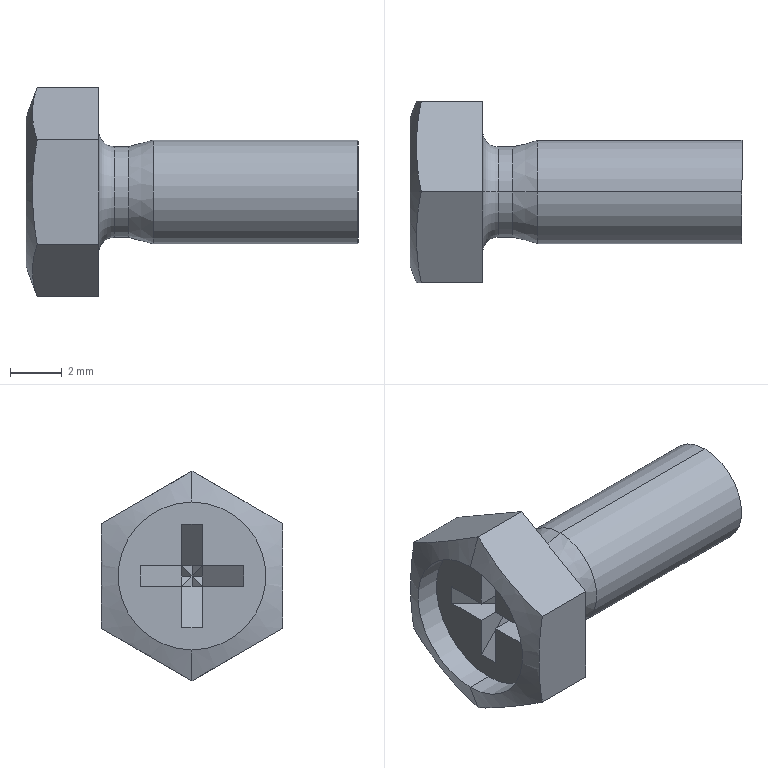Part | NX | features BREP 1 | 1 solid | 45 faces | box 12.8 x 7 x 8.083 mm | volume 207.191 mm3 | plane 33 | cylinder 6 | cone 4 | torus 2 | commonest cylinder face diameters 3.5 x2 4 x2 5.7 x2
STEP:
#1=CARTESIAN_POINT('',(1.,0.,-2.85));
#2=VERTEX_POINT('',#1);
#3=CARTESIAN_POINT('',(1.,0.,2.85));
#4=VERTEX_POINT('',#3);
#5=CARTESIAN_POINT('',(1.,0.,0.));
#6=DIRECTION('',(-1.,0.,0.));
#7=DIRECTION('',(0.,0.,1.));
#8=AXIS2_PLACEMENT_3D('',#5,#6,#7);
#9=CIRCLE('',#8,2.85);
#10=EDGE_CURVE('',#2,#4,#9,.T.);
#11=ORIENTED_EDGE('',*,*,#10,.F.);
#12=CARTESIAN_POINT('',(0.,0.,-2.85));
#13=VERTEX_POINT('',#12);
#14=CARTESIAN_POINT('',(1.,0.,-2.85));
#15=DIRECTION('',(-1.,0.,0.));
#16=VECTOR('',#15,1000.);
#17=LINE('',#14,#16);
#18=EDGE_CURVE('',#2,#13,#17,.T.);
#19=ORIENTED_EDGE('',*,*,#18,.T.);
#20=CARTESIAN_POINT('',(0.,0.,2.85));
#21=VERTEX_POINT('',#20);
#22=CARTESIAN_POINT('',(0.,0.,0.));
#23=DIRECTION('',(-1.,0.,0.));
#24=DIRECTION('',(0.,0.,1.));
#25=AXIS2_PLACEMENT_3D('',#22,#23,#24);
#26=CIRCLE('',#25,2.85);
#27=EDGE_CURVE('',#13,#21,#26,.T.);
#28=ORIENTED_EDGE('',*,*,#27,.T.);
#29=CARTESIAN_POINT('',(1.,0.,2.85));
#30=DIRECTION('',(-1.,0.,0.));
#31=VECTOR('',#30,1000.);
#32=LINE('',#29,#31);
#33=EDGE_CURVE('',#4,#21,#32,.T.);
#34=ORIENTED_EDGE('',*,*,#33,.F.);
#35=EDGE_LOOP('',(#11,#19,#28,#34));
#36=FACE_BOUND('',#35,.T.);
#37=CARTESIAN_POINT('',(1.,0.,0.));
#38=DIRECTION('',(-1.,0.,0.));
#39=DIRECTION('',(0.,0.,1.));
#40=AXIS2_PLACEMENT_3D('',#37,#38,#39);
#41=CYLINDRICAL_SURFACE('',#40,2.85);
#42=ADVANCED_FACE('',(#36),#41,.F.);
#43=CARTESIAN_POINT('',(1.,0.,0.));
#44=DIRECTION('',(-1.,0.,0.));
#45=DIRECTION('',(0.,0.,1.));
#46=AXIS2_PLACEMENT_3D('',#43,#44,#45);
#47=CIRCLE('',#46,2.85);
#48=EDGE_CURVE('',#4,#2,#47,.T.);
#49=ORIENTED_EDGE('',*,*,#48,.T.);
#50=ORIENTED_EDGE('',*,*,#10,.T.);
#51=EDGE_LOOP('',(#49,#50));
#52=FACE_BOUND('',#51,.T.);
#53=CARTESIAN_POINT('',(1.,2.,0.386));
#54=VERTEX_POINT('',#53);
#55=CARTESIAN_POINT('',(1.,2.,-0.386));
#56=VERTEX_POINT('',#55);
#57=CARTESIAN_POINT('',(1.,2.,0.));
#58=DIRECTION('',(0.,0.,-1.));
#59=VECTOR('',#58,1000.);
#60=LINE('',#57,#59);
#61=EDGE_CURVE('',#54,#56,#60,.T.);
#62=ORIENTED_EDGE('',*,*,#61,.F.);
#63=CARTESIAN_POINT('',(1.,0.386,0.386));
#64=VERTEX_POINT('',#63);
#65=CARTESIAN_POINT('',(1.,1.193,0.386));
#66=DIRECTION('',(0.,-1.,0.));
#67=VECTOR('',#66,1000.);
#68=LINE('',#65,#67);
#69=EDGE_CURVE('',#54,#64,#68,.T.);
#70=ORIENTED_EDGE('',*,*,#69,.T.);
#71=CARTESIAN_POINT('',(1.,0.386,2.));
#72=VERTEX_POINT('',#71);
#73=CARTESIAN_POINT('',(1.,0.386,1.193));
#74=DIRECTION('',(0.,0.,-1.));
#75=VECTOR('',#74,1000.);
#76=LINE('',#73,#75);
#77=EDGE_CURVE('',#72,#64,#76,.T.);
#78=ORIENTED_EDGE('',*,*,#77,.F.);
#79=CARTESIAN_POINT('',(1.,-0.386,2.));
#80=VERTEX_POINT('',#79);
#81=CARTESIAN_POINT('',(1.,0.,2.));
#82=DIRECTION('',(0.,1.,0.));
#83=VECTOR('',#82,1000.);
#84=LINE('',#81,#83);
#85=EDGE_CURVE('',#80,#72,#84,.T.);
#86=ORIENTED_EDGE('',*,*,#85,.F.);
#87=CARTESIAN_POINT('',(1.,-0.386,0.386));
#88=VERTEX_POINT('',#87);
#89=CARTESIAN_POINT('',(1.,-0.386,1.193));
#90=DIRECTION('',(0.,0.,-1.));
#91=VECTOR('',#90,1000.);
#92=LINE('',#89,#91);
#93=EDGE_CURVE('',#80,#88,#92,.T.);
#94=ORIENTED_EDGE('',*,*,#93,.T.);
#95=CARTESIAN_POINT('',(1.,-2.,0.386));
#96=VERTEX_POINT('',#95);
#97=CARTESIAN_POINT('',(1.,-1.193,0.386));
#98=DIRECTION('',(0.,-1.,0.));
#99=VECTOR('',#98,1000.);
#100=LINE('',#97,#99);
#101=EDGE_CURVE('',#88,#96,#100,.T.);
#102=ORIENTED_EDGE('',*,*,#101,.T.);
#103=CARTESIAN_POINT('',(1.,-2.,-0.386));
#104=VERTEX_POINT('',#103);
#105=CARTESIAN_POINT('',(1.,-2.,0.));
#106=DIRECTION('',(0.,0.,1.));
#107=VECTOR('',#106,1000.);
#108=LINE('',#105,#107);
#109=EDGE_CURVE('',#104,#96,#108,.T.);
#110=ORIENTED_EDGE('',*,*,#109,.F.);
#111=CARTESIAN_POINT('',(1.,-0.386,-0.386));
#112=VERTEX_POINT('',#111);
#113=CARTESIAN_POINT('',(1.,-1.193,-0.386));
#114=DIRECTION('',(0.,-1.,0.));
#115=VECTOR('',#114,1000.);
#116=LINE('',#113,#115);
#117=EDGE_CURVE('',#112,#104,#116,.T.);
#118=ORIENTED_EDGE('',*,*,#117,.F.);
#119=CARTESIAN_POINT('',(1.,-0.386,-2.));
#120=VERTEX_POINT('',#119);
#121=CARTESIAN_POINT('',(1.,-0.386,-1.193));
#122=DIRECTION('',(0.,0.,-1.));
#123=VECTOR('',#122,1000.);
#124=LINE('',#121,#123);
#125=EDGE_CURVE('',#112,#120,#124,.T.);
#126=ORIENTED_EDGE('',*,*,#125,.T.);
#127=CARTESIAN_POINT('',(1.,0.386,-2.));
#128=VERTEX_POINT('',#127);
#129=CARTESIAN_POINT('',(1.,0.,-2.));
#130=DIRECTION('',(0.,-1.,0.));
#131=VECTOR('',#130,1000.);
#132=LINE('',#129,#131);
#133=EDGE_CURVE('',#128,#120,#132,.T.);
#134=ORIENTED_EDGE('',*,*,#133,.F.);
#135=CARTESIAN_POINT('',(1.,0.386,-0.386));
#136=VERTEX_POINT('',#135);
#137=CARTESIAN_POINT('',(1.,0.386,-1.193));
#138=DIRECTION('',(0.,0.,-1.));
#139=VECTOR('',#138,1000.);
#140=LINE('',#137,#139);
#141=EDGE_CURVE('',#136,#128,#140,.T.);
#142=ORIENTED_EDGE('',*,*,#141,.F.);
#143=CARTESIAN_POINT('',(1.,1.193,-0.386));
#144=DIRECTION('',(0.,-1.,0.));
#145=VECTOR('',#144,1000.);
#146=LINE('',#143,#145);
#147=EDGE_CURVE('',#56,#136,#146,.T.);
#148=ORIENTED_EDGE('',*,*,#147,.F.);
#149=EDGE_LOOP('',(#62,#70,#78,#86,#94,#102,#110,#118,#126,#134,#142,#148));
#150=FACE_BOUND('',#149,.T.);
#151=CARTESIAN_POINT('',(1.,0.,0.));
#152=DIRECTION('',(-1.,0.,0.));
#153=DIRECTION('',(0.,0.,-1.));
#154=AXIS2_PLACEMENT_3D('',#151,#152,#153);
#155=PLANE('',#154);
#156=ADVANCED_FACE('',(#52,#150),#155,.T.);
#157=ORIENTED_EDGE('',*,*,#18,.F.);
#158=ORIENTED_EDGE('',*,*,#48,.F.);
#159=ORIENTED_EDGE('',*,*,#33,.T.);
#160=CARTESIAN_POINT('',(0.,0.,0.));
#161=DIRECTION('',(-1.,0.,0.));
#162=DIRECTION('',(0.,0.,1.));
#163=AXIS2_PLACEMENT_3D('',#160,#161,#162);
#164=CIRCLE('',#163,2.85);
#165=EDGE_CURVE('',#21,#13,#164,.T.);
#166=ORIENTED_EDGE('',*,*,#165,.T.);
#167=EDGE_LOOP('',(#157,#158,#159,#166));
#168=FACE_BOUND('',#167,.T.);
#169=CARTESIAN_POINT('',(1.,0.,0.));
#170=DIRECTION('',(-1.,0.,0.));
#171=DIRECTION('',(0.,0.,-1.));
#172=AXIS2_PLACEMENT_3D('',#169,#170,#171);
#173=CYLINDRICAL_SURFACE('',#172,2.85);
#174=ADVANCED_FACE('',(#168),#173,.F.);
#175=CARTESIAN_POINT('',(0.4337,0.000000012,4.041));
#176=VERTEX_POINT('',#175);
#177=CARTESIAN_POINT('',(171009.553,0.,469847.735));
#178=DIRECTION('',(0.342,0.,0.9397));
#179=VECTOR('',#178,1000.);
#180=LINE('',#177,#179);
#181=EDGE_CURVE('',#21,#176,#180,.T.);
#182=ORIENTED_EDGE('',*,*,#181,.F.);
#183=ORIENTED_EDGE('',*,*,#27,.F.);
#184=CARTESIAN_POINT('',(0.4337,0.000000012,-4.041));
#185=VERTEX_POINT('',#184);
#186=CARTESIAN_POINT('',(171009.553,0.,-469847.735));
#187=DIRECTION('',(0.342,0.,-0.9397));
#188=VECTOR('',#187,1000.);
#189=LINE('',#186,#188);
#190=EDGE_CURVE('',#13,#185,#189,.T.);
#191=ORIENTED_EDGE('',*,*,#190,.T.);
#192=CARTESIAN_POINT('',(0.4337,-3.5,-2.021));
#193=VERTEX_POINT('',#192);
#194=CARTESIAN_POINT('',(0.4337,-0.000000048,-4.041));
#195=CARTESIAN_POINT('',(0.1885,-1.167,-3.368));
#196=CARTESIAN_POINT('',(0.1885,-2.333,-2.694));
#197=CARTESIAN_POINT('',(0.4337,-3.5,-2.021));
#198=B_SPLINE_CURVE_WITH_KNOTS('',3,(#194,#195,#196,#197),.UNSPECIFIED.,.F.,.F.,(4,4),(0.,0.004041),.UNSPECIFIED.);
#199=EDGE_CURVE('',#185,#193,#198,.T.);
#200=ORIENTED_EDGE('',*,*,#199,.T.);
#201=CARTESIAN_POINT('',(0.4337,-3.5,2.021));
#202=VERTEX_POINT('',#201);
#203=CARTESIAN_POINT('',(0.4337,-3.5,-2.021));
#204=CARTESIAN_POINT('',(0.1885,-3.5,-0.6736));
#205=CARTESIAN_POINT('',(0.1885,-3.5,0.6736));
#206=CARTESIAN_POINT('',(0.4337,-3.5,2.021));
#207=B_SPLINE_CURVE_WITH_KNOTS('',3,(#203,#204,#205,#206),.UNSPECIFIED.,.F.,.F.,(4,4),(0.,0.004041),.UNSPECIFIED.);
#208=EDGE_CURVE('',#193,#202,#207,.T.);
#209=ORIENTED_EDGE('',*,*,#208,.T.);
#210=CARTESIAN_POINT('',(0.4337,-3.5,2.021));
#211=CARTESIAN_POINT('',(0.1885,-2.333,2.694));
#212=CARTESIAN_POINT('',(0.1885,-1.167,3.368));
#213=CARTESIAN_POINT('',(0.4337,-0.000000025,4.041));
#214=B_SPLINE_CURVE_WITH_KNOTS('',3,(#210,#211,#212,#213),.UNSPECIFIED.,.F.,.F.,(4,4),(0.,0.004041),.UNSPECIFIED.);
#215=EDGE_CURVE('',#202,#176,#214,.T.);
#216=ORIENTED_EDGE('',*,*,#215,.T.);
#217=EDGE_LOOP('',(#182,#183,#191,#200,#209,#216));
#218=FACE_BOUND('',#217,.T.);
#219=CARTESIAN_POINT('',(0.,0.,0.));
#220=DIRECTION('',(1.,0.,0.));
#221=DIRECTION('',(0.,0.,-1.));
#222=AXIS2_PLACEMENT_3D('',#219,#220,#221);
#223=CONICAL_SURFACE('',#222,2.85,1.222);
#224=ADVANCED_FACE('',(#218),#223,.T.);
#225=ORIENTED_EDGE('',*,*,#61,.T.);
#226=CARTESIAN_POINT('',(2.558,0.386,-0.386));
#227=VERTEX_POINT('',#226);
#228=CARTESIAN_POINT('',(1.779,1.193,-0.386));
#229=DIRECTION('',(0.6944,-0.7196,0.));
#230=VECTOR('',#229,1000.);
#231=LINE('',#228,#230);
#232=EDGE_CURVE('',#56,#227,#231,.T.);
#233=ORIENTED_EDGE('',*,*,#232,.T.);
#234=CARTESIAN_POINT('',(2.558,0.386,0.386));
#235=VERTEX_POINT('',#234);
#236=CARTESIAN_POINT('',(2.558,0.386,0.));
#237=DIRECTION('',(0.,0.,-1.));
#238=VECTOR('',#237,1000.);
#239=LINE('',#236,#238);
#240=EDGE_CURVE('',#235,#227,#239,.T.);
#241=ORIENTED_EDGE('',*,*,#240,.F.);
#242=CARTESIAN_POINT('',(1.779,1.193,0.386));
#243=DIRECTION('',(0.6944,-0.7196,0.));
#244=VECTOR('',#243,1000.);
#245=LINE('',#242,#244);
#246=EDGE_CURVE('',#54,#235,#245,.T.);
#247=ORIENTED_EDGE('',*,*,#246,.F.);
#248=EDGE_LOOP('',(#225,#233,#241,#247));
#249=FACE_BOUND('',#248,.T.);
#250=CARTESIAN_POINT('',(0.5,2.518,0.386));
#251=DIRECTION('',(0.7196,0.6944,0.));
#252=DIRECTION('',(0.6944,-0.7196,0.));
#253=AXIS2_PLACEMENT_3D('',#250,#251,#252);
#254=PLANE('',#253);
#255=ADVANCED_FACE('',(#249),#254,.F.);
#256=ORIENTED_EDGE('',*,*,#246,.T.);
#257=CARTESIAN_POINT('',(1.779,0.386,0.386));
#258=DIRECTION('',(-1.,0.,0.));
#259=VECTOR('',#258,1000.);
#260=LINE('',#257,#259);
#261=EDGE_CURVE('',#235,#64,#260,.T.);
#262=ORIENTED_EDGE('',*,*,#261,.T.);
#263=ORIENTED_EDGE('',*,*,#69,.F.);
#264=EDGE_LOOP('',(#256,#262,#263));
#265=FACE_BOUND('',#264,.T.);
#266=CARTESIAN_POINT('',(2.93,0.,0.386));
#267=DIRECTION('',(0.,0.,-1.));
#268=DIRECTION('',(0.,-1.,0.));
#269=AXIS2_PLACEMENT_3D('',#266,#267,#268);
#270=PLANE('',#269);
#271=ADVANCED_FACE('',(#265),#270,.T.);
#272=ORIENTED_EDGE('',*,*,#261,.F.);
#273=CARTESIAN_POINT('',(1.779,0.386,1.193));
#274=DIRECTION('',(0.6944,0.,-0.7196));
#275=VECTOR('',#274,1000.);
#276=LINE('',#273,#275);
#277=EDGE_CURVE('',#72,#235,#276,.T.);
#278=ORIENTED_EDGE('',*,*,#277,.F.);
#279=ORIENTED_EDGE('',*,*,#77,.T.);
#280=EDGE_LOOP('',(#272,#278,#279));
#281=FACE_BOUND('',#280,.T.);
#282=CARTESIAN_POINT('',(2.93,0.386,0.));
#283=DIRECTION('',(0.,1.,0.));
#284=DIRECTION('',(0.,0.,-1.));
#285=AXIS2_PLACEMENT_3D('',#282,#283,#284);
#286=PLANE('',#285);
#287=ADVANCED_FACE('',(#281),#286,.F.);
#288=CARTESIAN_POINT('',(2.558,-0.386,0.386));
#289=VERTEX_POINT('',#288);
#290=CARTESIAN_POINT('',(2.558,0.,0.386));
#291=DIRECTION('',(0.,1.,0.));
#292=VECTOR('',#291,1000.);
#293=LINE('',#290,#292);
#294=EDGE_CURVE('',#289,#235,#293,.T.);
#295=ORIENTED_EDGE('',*,*,#294,.F.);
#296=CARTESIAN_POINT('',(1.779,-0.386,1.193));
#297=DIRECTION('',(0.6944,0.,-0.7196));
#298=VECTOR('',#297,1000.);
#299=LINE('',#296,#298);
#300=EDGE_CURVE('',#80,#289,#299,.T.);
#301=ORIENTED_EDGE('',*,*,#300,.F.);
#302=ORIENTED_EDGE('',*,*,#85,.T.);
#303=ORIENTED_EDGE('',*,*,#277,.T.);
#304=EDGE_LOOP('',(#295,#301,#302,#303));
#305=FACE_BOUND('',#304,.T.);
#306=CARTESIAN_POINT('',(0.5,-0.386,2.518));
#307=DIRECTION('',(0.7196,0.,0.6944));
#308=DIRECTION('',(-0.6944,0.,0.7196));
#309=AXIS2_PLACEMENT_3D('',#306,#307,#308);
#310=PLANE('',#309);
#311=ADVANCED_FACE('',(#305),#310,.F.);
#312=ORIENTED_EDGE('',*,*,#300,.T.);
#313=CARTESIAN_POINT('',(1.779,-0.386,0.386));
#314=DIRECTION('',(-1.,0.,0.));
#315=VECTOR('',#314,1000.);
#316=LINE('',#313,#315);
#317=EDGE_CURVE('',#289,#88,#316,.T.);
#318=ORIENTED_EDGE('',*,*,#317,.T.);
#319=ORIENTED_EDGE('',*,*,#93,.F.);
#320=EDGE_LOOP('',(#312,#318,#319));
#321=FACE_BOUND('',#320,.T.);
#322=CARTESIAN_POINT('',(2.93,-0.386,0.));
#323=DIRECTION('',(0.,1.,0.));
#324=DIRECTION('',(0.,0.,-1.));
#325=AXIS2_PLACEMENT_3D('',#322,#323,#324);
#326=PLANE('',#325);
#327=ADVANCED_FACE('',(#321),#326,.T.);
#328=ORIENTED_EDGE('',*,*,#317,.F.);
#329=CARTESIAN_POINT('',(1.779,-1.193,0.386));
#330=DIRECTION('',(-0.6944,-0.7196,0.));
#331=VECTOR('',#330,1000.);
#332=LINE('',#329,#331);
#333=EDGE_CURVE('',#289,#96,#332,.T.);
#334=ORIENTED_EDGE('',*,*,#333,.T.);
#335=ORIENTED_EDGE('',*,*,#101,.F.);
#336=EDGE_LOOP('',(#328,#334,#335));
#337=FACE_BOUND('',#336,.T.);
#338=CARTESIAN_POINT('',(2.93,0.,0.386));
#339=DIRECTION('',(0.,0.,-1.));
#340=DIRECTION('',(0.,-1.,0.));
#341=AXIS2_PLACEMENT_3D('',#338,#339,#340);
#342=PLANE('',#341);
#343=ADVANCED_FACE('',(#337),#342,.T.);
#344=ORIENTED_EDGE('',*,*,#109,.T.);
#345=ORIENTED_EDGE('',*,*,#333,.F.);
#346=CARTESIAN_POINT('',(2.558,-0.386,-0.386));
#347=VERTEX_POINT('',#346);
#348=CARTESIAN_POINT('',(2.558,-0.386,0.));
#349=DIRECTION('',(0.,0.,-1.));
#350=VECTOR('',#349,1000.);
#351=LINE('',#348,#350);
#352=EDGE_CURVE('',#289,#347,#351,.T.);
#353=ORIENTED_EDGE('',*,*,#352,.T.);
#354=CARTESIAN_POINT('',(1.779,-1.193,-0.386));
#355=DIRECTION('',(-0.6944,-0.7196,0.));
#356=VECTOR('',#355,1000.);
#357=LINE('',#354,#356);
#358=EDGE_CURVE('',#347,#104,#357,.T.);
#359=ORIENTED_EDGE('',*,*,#358,.T.);
#360=EDGE_LOOP('',(#344,#345,#353,#359));
#361=FACE_BOUND('',#360,.T.);
#362=CARTESIAN_POINT('',(2.93,0.,0.386));
#363=DIRECTION('',(0.7196,-0.6944,0.));
#364=DIRECTION('',(-0.6944,-0.7196,0.));
#365=AXIS2_PLACEMENT_3D('',#362,#363,#364);
#366=PLANE('',#365);
#367=ADVANCED_FACE('',(#361),#366,.F.);
#368=ORIENTED_EDGE('',*,*,#117,.T.);
#369=ORIENTED_EDGE('',*,*,#358,.F.);
#370=CARTESIAN_POINT('',(1.779,-0.386,-0.386));
#371=DIRECTION('',(-1.,0.,0.));
#372=VECTOR('',#371,1000.);
#373=LINE('',#370,#372);
#374=EDGE_CURVE('',#347,#112,#373,.T.);
#375=ORIENTED_EDGE('',*,*,#374,.T.);
#376=EDGE_LOOP('',(#368,#369,#375));
#377=FACE_BOUND('',#376,.T.);
#378=CARTESIAN_POINT('',(2.93,0.,-0.386));
#379=DIRECTION('',(0.,0.,-1.));
#380=DIRECTION('',(0.,-1.,0.));
#381=AXIS2_PLACEMENT_3D('',#378,#379,#380);
#382=PLANE('',#381);
#383=ADVANCED_FACE('',(#377),#382,.F.);
#384=ORIENTED_EDGE('',*,*,#374,.F.);
#385=CARTESIAN_POINT('',(1.779,-0.386,-1.193));
#386=DIRECTION('',(-0.6944,0.,-0.7196));
#387=VECTOR('',#386,1000.);
#388=LINE('',#385,#387);
#389=EDGE_CURVE('',#347,#120,#388,.T.);
#390=ORIENTED_EDGE('',*,*,#389,.T.);
#391=ORIENTED_EDGE('',*,*,#125,.F.);
#392=EDGE_LOOP('',(#384,#390,#391));
#393=FACE_BOUND('',#392,.T.);
#394=CARTESIAN_POINT('',(2.93,-0.386,0.));
#395=DIRECTION('',(0.,1.,0.));
#396=DIRECTION('',(0.,0.,-1.));
#397=AXIS2_PLACEMENT_3D('',#394,#395,#396);
#398=PLANE('',#397);
#399=ADVANCED_FACE('',(#393),#398,.T.);
#400=ORIENTED_EDGE('',*,*,#389,.F.);
#401=CARTESIAN_POINT('',(2.558,0.,-0.386));
#402=DIRECTION('',(0.,1.,0.));
#403=VECTOR('',#402,1000.);
#404=LINE('',#401,#403);
#405=EDGE_CURVE('',#347,#227,#404,.T.);
#406=ORIENTED_EDGE('',*,*,#405,.T.);
#407=CARTESIAN_POINT('',(1.779,0.386,-1.193));
#408=DIRECTION('',(-0.6944,0.,-0.7196));
#409=VECTOR('',#408,1000.);
#410=LINE('',#407,#409);
#411=EDGE_CURVE('',#227,#128,#410,.T.);
#412=ORIENTED_EDGE('',*,*,#411,.T.);
#413=ORIENTED_EDGE('',*,*,#133,.T.);
#414=EDGE_LOOP('',(#400,#406,#412,#413));
#415=FACE_BOUND('',#414,.T.);
#416=CARTESIAN_POINT('',(2.93,-0.386,0.));
#417=DIRECTION('',(0.7196,0.,-0.6944));
#418=DIRECTION('',(0.6944,0.,0.7196));
#419=AXIS2_PLACEMENT_3D('',#416,#417,#418);
#420=PLANE('',#419);
#421=ADVANCED_FACE('',(#415),#420,.F.);
#422=ORIENTED_EDGE('',*,*,#411,.F.);
#423=CARTESIAN_POINT('',(1.779,0.386,-0.386));
#424=DIRECTION('',(-1.,0.,0.));
#425=VECTOR('',#424,1000.);
#426=LINE('',#423,#425);
#427=EDGE_CURVE('',#227,#136,#426,.T.);
#428=ORIENTED_EDGE('',*,*,#427,.T.);
#429=ORIENTED_EDGE('',*,*,#141,.T.);
#430=EDGE_LOOP('',(#422,#428,#429));
#431=FACE_BOUND('',#430,.T.);
#432=CARTESIAN_POINT('',(2.93,0.386,0.));
#433=DIRECTION('',(0.,1.,0.));
#434=DIRECTION('',(0.,0.,-1.));
#435=AXIS2_PLACEMENT_3D('',#432,#433,#434);
#436=PLANE('',#435);
#437=ADVANCED_FACE('',(#431),#436,.F.);
#438=ORIENTED_EDGE('',*,*,#147,.T.);
#439=ORIENTED_EDGE('',*,*,#427,.F.);
#440=ORIENTED_EDGE('',*,*,#232,.F.);
#441=EDGE_LOOP('',(#438,#439,#440));
#442=FACE_BOUND('',#441,.T.);
#443=CARTESIAN_POINT('',(2.93,0.,-0.386));
#444=DIRECTION('',(0.,0.,-1.));
#445=DIRECTION('',(0.,-1.,0.));
#446=AXIS2_PLACEMENT_3D('',#443,#444,#445);
#447=PLANE('',#446);
#448=ADVANCED_FACE('',(#442),#447,.F.);
#449=ORIENTED_EDGE('',*,*,#165,.F.);
#450=ORIENTED_EDGE('',*,*,#181,.T.);
#451=CARTESIAN_POINT('',(0.4337,3.5,2.021));
#452=VERTEX_POINT('',#451);
#453=CARTESIAN_POINT('',(0.4337,0.000000059,4.041));
#454=CARTESIAN_POINT('',(0.1885,1.167,3.368));
#455=CARTESIAN_POINT('',(0.1885,2.333,2.694));
#456=CARTESIAN_POINT('',(0.4337,3.5,2.021));
#457=B_SPLINE_CURVE_WITH_KNOTS('',3,(#453,#454,#455,#456),.UNSPECIFIED.,.F.,.F.,(4,4),(0.,0.004041),.UNSPECIFIED.);
#458=EDGE_CURVE('',#176,#452,#457,.T.);
#459=ORIENTED_EDGE('',*,*,#458,.T.);
#460=CARTESIAN_POINT('',(0.4337,3.5,-2.021));
#461=VERTEX_POINT('',#460);
#462=CARTESIAN_POINT('',(0.4337,3.5,2.021));
#463=CARTESIAN_POINT('',(0.1885,3.5,0.6736));
#464=CARTESIAN_POINT('',(0.1885,3.5,-0.6736));
#465=CARTESIAN_POINT('',(0.4337,3.5,-2.021));
#466=B_SPLINE_CURVE_WITH_KNOTS('',3,(#462,#463,#464,#465),.UNSPECIFIED.,.F.,.F.,(4,4),(0.,0.004041),.UNSPECIFIED.);
#467=EDGE_CURVE('',#452,#461,#466,.T.);
#468=ORIENTED_EDGE('',*,*,#467,.T.);
#469=CARTESIAN_POINT('',(0.4337,3.5,-2.021));
#470=CARTESIAN_POINT('',(0.1885,2.333,-2.694));
#471=CARTESIAN_POINT('',(0.1885,1.167,-3.368));
#472=CARTESIAN_POINT('',(0.4337,0.000000003,-4.041));
#473=B_SPLINE_CURVE_WITH_KNOTS('',3,(#469,#470,#471,#472),.UNSPECIFIED.,.F.,.F.,(4,4),(0.,0.004041),.UNSPECIFIED.);
#474=EDGE_CURVE('',#461,#185,#473,.T.);
#475=ORIENTED_EDGE('',*,*,#474,.T.);
#476=ORIENTED_EDGE('',*,*,#190,.F.);
#477=EDGE_LOOP('',(#449,#450,#459,#468,#475,#476));
#478=FACE_BOUND('',#477,.T.);
#479=CARTESIAN_POINT('',(0.,0.,0.));
#480=DIRECTION('',(1.,0.,0.));
#481=DIRECTION('',(0.,0.,1.));
#482=AXIS2_PLACEMENT_3D('',#479,#480,#481);
#483=CONICAL_SURFACE('',#482,2.85,1.222);
#484=ADVANCED_FACE('',(#478),#483,.T.);
#485=ORIENTED_EDGE('',*,*,#199,.F.);
#486=CARTESIAN_POINT('',(2.8,0.,-4.041));
#487=VERTEX_POINT('',#486);
#488=CARTESIAN_POINT('',(1.617,0.,-4.041));
#489=DIRECTION('',(-1.,0.,0.));
#490=VECTOR('',#489,1000.);
#491=LINE('',#488,#490);
#492=EDGE_CURVE('',#487,#185,#491,.T.);
#493=ORIENTED_EDGE('',*,*,#492,.F.);
#494=CARTESIAN_POINT('',(2.8,-3.5,-2.021));
#495=VERTEX_POINT('',#494);
#496=CARTESIAN_POINT('',(2.8,-1.75,-3.031));
#497=DIRECTION('',(0.,0.866,-0.5));
#498=VECTOR('',#497,1000.);
#499=LINE('',#496,#498);
#500=EDGE_CURVE('',#495,#487,#499,.T.);
#501=ORIENTED_EDGE('',*,*,#500,.F.);
#502=CARTESIAN_POINT('',(1.617,-3.5,-2.021));
#503=DIRECTION('',(-1.,0.,0.));
#504=VECTOR('',#503,1000.);
#505=LINE('',#502,#504);
#506=EDGE_CURVE('',#495,#193,#505,.T.);
#507=ORIENTED_EDGE('',*,*,#506,.T.);
#508=EDGE_LOOP('',(#485,#493,#501,#507));
#509=FACE_BOUND('',#508,.T.);
#510=CARTESIAN_POINT('',(2.8,-3.5,-2.021));
#511=DIRECTION('',(0.,0.5,0.866));
#512=DIRECTION('',(0.,0.866,-0.5));
#513=AXIS2_PLACEMENT_3D('',#510,#511,#512);
#514=PLANE('',#513);
#515=ADVANCED_FACE('',(#509),#514,.F.);
#516=ORIENTED_EDGE('',*,*,#208,.F.);
#517=ORIENTED_EDGE('',*,*,#506,.F.);
#518=CARTESIAN_POINT('',(2.8,-3.5,2.021));
#519=VERTEX_POINT('',#518);
#520=CARTESIAN_POINT('',(2.8,-3.5,0.));
#521=DIRECTION('',(0.,0.,-1.));
#522=VECTOR('',#521,1000.);
#523=LINE('',#520,#522);
#524=EDGE_CURVE('',#519,#495,#523,.T.);
#525=ORIENTED_EDGE('',*,*,#524,.F.);
#526=CARTESIAN_POINT('',(1.617,-3.5,2.021));
#527=DIRECTION('',(-1.,0.,0.));
#528=VECTOR('',#527,1000.);
#529=LINE('',#526,#528);
#530=EDGE_CURVE('',#519,#202,#529,.T.);
#531=ORIENTED_EDGE('',*,*,#530,.T.);
#532=EDGE_LOOP('',(#516,#517,#525,#531));
#533=FACE_BOUND('',#532,.T.);
#534=CARTESIAN_POINT('',(2.8,-3.5,2.021));
#535=DIRECTION('',(0.,1.,0.));
#536=DIRECTION('',(0.,0.,-1.));
#537=AXIS2_PLACEMENT_3D('',#534,#535,#536);
#538=PLANE('',#537);
#539=ADVANCED_FACE('',(#533),#538,.F.);
#540=ORIENTED_EDGE('',*,*,#215,.F.);
#541=ORIENTED_EDGE('',*,*,#530,.F.);
#542=CARTESIAN_POINT('',(2.8,0.,4.041));
#543=VERTEX_POINT('',#542);
#544=CARTESIAN_POINT('',(2.8,-1.75,3.031));
#545=DIRECTION('',(0.,-0.866,-0.5));
#546=VECTOR('',#545,1000.);
#547=LINE('',#544,#546);
#548=EDGE_CURVE('',#543,#519,#547,.T.);
#549=ORIENTED_EDGE('',*,*,#548,.F.);
#550=CARTESIAN_POINT('',(1.617,0.,4.041));
#551=DIRECTION('',(-1.,0.,0.));
#552=VECTOR('',#551,1000.);
#553=LINE('',#550,#552);
#554=EDGE_CURVE('',#543,#176,#553,.T.);
#555=ORIENTED_EDGE('',*,*,#554,.T.);
#556=EDGE_LOOP('',(#540,#541,#549,#555));
#557=FACE_BOUND('',#556,.T.);
#558=CARTESIAN_POINT('',(2.8,0.,4.041));
#559=DIRECTION('',(0.,0.5,-0.866));
#560=DIRECTION('',(0.,-0.866,-0.5));
#561=AXIS2_PLACEMENT_3D('',#558,#559,#560);
#562=PLANE('',#561);
#563=ADVANCED_FACE('',(#557),#562,.F.);
#564=CARTESIAN_POINT('',(2.93,0.386,0.));
#565=VERTEX_POINT('',#564);
#566=CARTESIAN_POINT('',(2.744,0.386,0.193));
#567=DIRECTION('',(0.6944,0.,-0.7196));
#568=VECTOR('',#567,1000.);
#569=LINE('',#566,#568);
#570=EDGE_CURVE('',#235,#565,#569,.T.);
#571=ORIENTED_EDGE('',*,*,#570,.F.);
#572=ORIENTED_EDGE('',*,*,#240,.T.);
#573=CARTESIAN_POINT('',(2.744,0.386,-0.193));
#574=DIRECTION('',(-0.6944,0.,-0.7196));
#575=VECTOR('',#574,1000.);
#576=LINE('',#573,#575);
#577=EDGE_CURVE('',#565,#227,#576,.T.);
#578=ORIENTED_EDGE('',*,*,#577,.F.);
#579=EDGE_LOOP('',(#571,#572,#578));
#580=FACE_BOUND('',#579,.T.);
#581=CARTESIAN_POINT('',(2.93,0.386,0.));
#582=DIRECTION('',(0.,1.,0.));
#583=DIRECTION('',(0.,0.,-1.));
#584=AXIS2_PLACEMENT_3D('',#581,#582,#583);
#585=PLANE('',#584);
#586=ADVANCED_FACE('',(#580),#585,.F.);
#587=ORIENTED_EDGE('',*,*,#294,.T.);
#588=CARTESIAN_POINT('',(2.93,0.,0.386));
#589=VERTEX_POINT('',#588);
#590=CARTESIAN_POINT('',(2.744,0.193,0.386));
#591=DIRECTION('',(0.6944,-0.7196,0.));
#592=VECTOR('',#591,1000.);
#593=LINE('',#590,#592);
#594=EDGE_CURVE('',#235,#589,#593,.T.);
#595=ORIENTED_EDGE('',*,*,#594,.T.);
#596=CARTESIAN_POINT('',(2.744,-0.193,0.386));
#597=DIRECTION('',(-0.6944,-0.7196,0.));
#598=VECTOR('',#597,1000.);
#599=LINE('',#596,#598);
#600=EDGE_CURVE('',#589,#289,#599,.T.);
#601=ORIENTED_EDGE('',*,*,#600,.T.);
#602=EDGE_LOOP('',(#587,#595,#601));
#603=FACE_BOUND('',#602,.T.);
#604=CARTESIAN_POINT('',(2.93,0.,0.386));
#605=DIRECTION('',(0.,0.,-1.));
#606=DIRECTION('',(0.,-1.,0.));
#607=AXIS2_PLACEMENT_3D('',#604,#605,#606);
#608=PLANE('',#607);
#609=ADVANCED_FACE('',(#603),#608,.T.);
#610=ORIENTED_EDGE('',*,*,#352,.F.);
#611=CARTESIAN_POINT('',(2.93,-0.386,0.));
#612=VERTEX_POINT('',#611);
#613=CARTESIAN_POINT('',(2.744,-0.386,0.193));
#614=DIRECTION('',(0.6944,0.,-0.7196));
#615=VECTOR('',#614,1000.);
#616=LINE('',#613,#615);
#617=EDGE_CURVE('',#289,#612,#616,.T.);
#618=ORIENTED_EDGE('',*,*,#617,.T.);
#619=CARTESIAN_POINT('',(2.744,-0.386,-0.193));
#620=DIRECTION('',(-0.6944,0.,-0.7196));
#621=VECTOR('',#620,1000.);
#622=LINE('',#619,#621);
#623=EDGE_CURVE('',#612,#347,#622,.T.);
#624=ORIENTED_EDGE('',*,*,#623,.T.);
#625=EDGE_LOOP('',(#610,#618,#624));
#626=FACE_BOUND('',#625,.T.);
#627=CARTESIAN_POINT('',(2.93,-0.386,0.));
#628=DIRECTION('',(0.,1.,0.));
#629=DIRECTION('',(0.,0.,-1.));
#630=AXIS2_PLACEMENT_3D('',#627,#628,#629);
#631=PLANE('',#630);
#632=ADVANCED_FACE('',(#626),#631,.T.);
#633=CARTESIAN_POINT('',(2.93,0.,-0.386));
#634=VERTEX_POINT('',#633);
#635=CARTESIAN_POINT('',(2.744,-0.193,-0.386));
#636=DIRECTION('',(-0.6944,-0.7196,0.));
#637=VECTOR('',#636,1000.);
#638=LINE('',#635,#637);
#639=EDGE_CURVE('',#634,#347,#638,.T.);
#640=ORIENTED_EDGE('',*,*,#639,.F.);
#641=CARTESIAN_POINT('',(2.744,0.193,-0.386));
#642=DIRECTION('',(0.6944,-0.7196,0.));
#643=VECTOR('',#642,1000.);
#644=LINE('',#641,#643);
#645=EDGE_CURVE('',#227,#634,#644,.T.);
#646=ORIENTED_EDGE('',*,*,#645,.F.);
#647=ORIENTED_EDGE('',*,*,#405,.F.);
#648=EDGE_LOOP('',(#640,#646,#647));
#649=FACE_BOUND('',#648,.T.);
#650=CARTESIAN_POINT('',(2.93,0.,-0.386));
#651=DIRECTION('',(0.,0.,-1.));
#652=DIRECTION('',(0.,-1.,0.));
#653=AXIS2_PLACEMENT_3D('',#650,#651,#652);
#654=PLANE('',#653);
#655=ADVANCED_FACE('',(#649),#654,.F.);
#656=ORIENTED_EDGE('',*,*,#458,.F.);
#657=ORIENTED_EDGE('',*,*,#554,.F.);
#658=CARTESIAN_POINT('',(2.8,3.5,2.021));
#659=VERTEX_POINT('',#658);
#660=CARTESIAN_POINT('',(2.8,1.75,3.031));
#661=DIRECTION('',(0.,-0.866,0.5));
#662=VECTOR('',#661,1000.);
#663=LINE('',#660,#662);
#664=EDGE_CURVE('',#659,#543,#663,.T.);
#665=ORIENTED_EDGE('',*,*,#664,.F.);
#666=CARTESIAN_POINT('',(1.617,3.5,2.021));
#667=DIRECTION('',(-1.,0.,0.));
#668=VECTOR('',#667,1000.);
#669=LINE('',#666,#668);
#670=EDGE_CURVE('',#659,#452,#669,.T.);
#671=ORIENTED_EDGE('',*,*,#670,.T.);
#672=EDGE_LOOP('',(#656,#657,#665,#671));
#673=FACE_BOUND('',#672,.T.);
#674=CARTESIAN_POINT('',(2.8,3.5,2.021));
#675=DIRECTION('',(0.,-0.5,-0.866));
#676=DIRECTION('',(0.,-0.866,0.5));
#677=AXIS2_PLACEMENT_3D('',#674,#675,#676);
#678=PLANE('',#677);
#679=ADVANCED_FACE('',(#673),#678,.F.);
#680=ORIENTED_EDGE('',*,*,#467,.F.);
#681=ORIENTED_EDGE('',*,*,#670,.F.);
#682=CARTESIAN_POINT('',(2.8,3.5,-2.021));
#683=VERTEX_POINT('',#682);
#684=CARTESIAN_POINT('',(2.8,3.5,0.));
#685=DIRECTION('',(0.,0.,1.));
#686=VECTOR('',#685,1000.);
#687=LINE('',#684,#686);
#688=EDGE_CURVE('',#683,#659,#687,.T.);
#689=ORIENTED_EDGE('',*,*,#688,.F.);
#690=CARTESIAN_POINT('',(1.617,3.5,-2.021));
#691=DIRECTION('',(-1.,0.,0.));
#692=VECTOR('',#691,1000.);
#693=LINE('',#690,#692);
#694=EDGE_CURVE('',#683,#461,#693,.T.);
#695=ORIENTED_EDGE('',*,*,#694,.T.);
#696=EDGE_LOOP('',(#680,#681,#689,#695));
#697=FACE_BOUND('',#696,.T.);
#698=CARTESIAN_POINT('',(2.8,3.5,-2.021));
#699=DIRECTION('',(0.,-1.,0.));
#700=DIRECTION('',(0.,0.,1.));
#701=AXIS2_PLACEMENT_3D('',#698,#699,#700);
#702=PLANE('',#701);
#703=ADVANCED_FACE('',(#697),#702,.F.);
#704=ORIENTED_EDGE('',*,*,#474,.F.);
#705=ORIENTED_EDGE('',*,*,#694,.F.);
#706=CARTESIAN_POINT('',(2.8,1.75,-3.031));
#707=DIRECTION('',(0.,0.866,0.5));
#708=VECTOR('',#707,1000.);
#709=LINE('',#706,#708);
#710=EDGE_CURVE('',#487,#683,#709,.T.);
#711=ORIENTED_EDGE('',*,*,#710,.F.);
#712=ORIENTED_EDGE('',*,*,#492,.T.);
#713=EDGE_LOOP('',(#704,#705,#711,#712));
#714=FACE_BOUND('',#713,.T.);
#715=CARTESIAN_POINT('',(2.8,0.,-4.041));
#716=DIRECTION('',(0.,-0.5,0.866));
#717=DIRECTION('',(0.,0.866,0.5));
#718=AXIS2_PLACEMENT_3D('',#715,#716,#717);
#719=PLANE('',#718);
#720=ADVANCED_FACE('',(#714),#719,.F.);
#721=ORIENTED_EDGE('',*,*,#524,.T.);
#722=ORIENTED_EDGE('',*,*,#500,.T.);
#723=ORIENTED_EDGE('',*,*,#710,.T.);
#724=ORIENTED_EDGE('',*,*,#688,.T.);
#725=ORIENTED_EDGE('',*,*,#664,.T.);
#726=ORIENTED_EDGE('',*,*,#548,.T.);
#727=EDGE_LOOP('',(#721,#722,#723,#724,#725,#726));
#728=FACE_BOUND('',#727,.T.);
#729=CARTESIAN_POINT('',(2.8,0.,2.35));
#730=VERTEX_POINT('',#729);
#731=CARTESIAN_POINT('',(2.8,0.,-2.35));
#732=VERTEX_POINT('',#731);
#733=CARTESIAN_POINT('',(2.8,-0.000000001,0.));
#734=DIRECTION('',(-1.,0.,0.));
#735=DIRECTION('',(0.,0.,1.));
#736=AXIS2_PLACEMENT_3D('',#733,#734,#735);
#737=CIRCLE('',#736,2.35);
#738=EDGE_CURVE('',#730,#732,#737,.T.);
#739=ORIENTED_EDGE('',*,*,#738,.T.);
#740=CARTESIAN_POINT('',(2.8,0.000000001,0.));
#741=DIRECTION('',(-1.,0.,0.));
#742=DIRECTION('',(0.,0.,1.));
#743=AXIS2_PLACEMENT_3D('',#740,#741,#742);
#744=CIRCLE('',#743,2.35);
#745=EDGE_CURVE('',#732,#730,#744,.T.);
#746=ORIENTED_EDGE('',*,*,#745,.T.);
#747=EDGE_LOOP('',(#739,#746));
#748=FACE_BOUND('',#747,.T.);
#749=CARTESIAN_POINT('',(2.8,-3.5,2.021));
#750=DIRECTION('',(-1.,0.,0.));
#751=DIRECTION('',(0.,0.,-1.));
#752=AXIS2_PLACEMENT_3D('',#749,#750,#751);
#753=PLANE('',#752);
#754=ADVANCED_FACE('',(#728,#748),#753,.F.);
#755=CARTESIAN_POINT('',(2.93,0.,0.));
#756=VERTEX_POINT('',#755);
#757=CARTESIAN_POINT('',(2.93,0.193,0.));
#758=DIRECTION('',(0.,1.,0.));
#759=VECTOR('',#758,1000.);
#760=LINE('',#757,#759);
#761=EDGE_CURVE('',#756,#565,#760,.T.);
#762=ORIENTED_EDGE('',*,*,#761,.F.);
#763=CARTESIAN_POINT('',(2.744,0.193,0.193));
#764=DIRECTION('',(-0.5636,0.5841,0.5841));
#765=VECTOR('',#764,1000.);
#766=LINE('',#763,#765);
#767=EDGE_CURVE('',#756,#235,#766,.T.);
#768=ORIENTED_EDGE('',*,*,#767,.T.);
#769=ORIENTED_EDGE('',*,*,#570,.T.);
#770=EDGE_LOOP('',(#762,#768,#769));
#771=FACE_BOUND('',#770,.T.);
#772=CARTESIAN_POINT('',(0.5,-0.386,2.518));
#773=DIRECTION('',(0.7196,0.,0.6944));
#774=DIRECTION('',(-0.6944,0.,0.7196));
#775=AXIS2_PLACEMENT_3D('',#772,#773,#774);
#776=PLANE('',#775);
#777=ADVANCED_FACE('',(#771),#776,.F.);
#778=ORIENTED_EDGE('',*,*,#577,.T.);
#779=CARTESIAN_POINT('',(2.744,0.193,-0.193));
#780=DIRECTION('',(0.5636,-0.5841,0.5841));
#781=VECTOR('',#780,1000.);
#782=LINE('',#779,#781);
#783=EDGE_CURVE('',#227,#756,#782,.T.);
#784=ORIENTED_EDGE('',*,*,#783,.T.);
#785=ORIENTED_EDGE('',*,*,#761,.T.);
#786=EDGE_LOOP('',(#778,#784,#785));
#787=FACE_BOUND('',#786,.T.);
#788=CARTESIAN_POINT('',(2.93,-0.386,0.));
#789=DIRECTION('',(0.7196,0.,-0.6944));
#790=DIRECTION('',(0.6944,0.,0.7196));
#791=AXIS2_PLACEMENT_3D('',#788,#789,#790);
#792=PLANE('',#791);
#793=ADVANCED_FACE('',(#787),#792,.F.);
#794=CARTESIAN_POINT('',(2.93,0.,0.193));
#795=DIRECTION('',(0.,0.,-1.));
#796=VECTOR('',#795,1000.);
#797=LINE('',#794,#796);
#798=EDGE_CURVE('',#589,#756,#797,.T.);
#799=ORIENTED_EDGE('',*,*,#798,.F.);
#800=ORIENTED_EDGE('',*,*,#594,.F.);
#801=ORIENTED_EDGE('',*,*,#767,.F.);
#802=EDGE_LOOP('',(#799,#800,#801));
#803=FACE_BOUND('',#802,.T.);
#804=CARTESIAN_POINT('',(0.5,2.518,0.386));
#805=DIRECTION('',(0.7196,0.6944,0.));
#806=DIRECTION('',(0.6944,-0.7196,0.));
#807=AXIS2_PLACEMENT_3D('',#804,#805,#806);
#808=PLANE('',#807);
#809=ADVANCED_FACE('',(#803),#808,.F.);
#810=ORIENTED_EDGE('',*,*,#600,.F.);
#811=ORIENTED_EDGE('',*,*,#798,.T.);
#812=CARTESIAN_POINT('',(2.744,-0.193,0.193));
#813=DIRECTION('',(0.5636,0.5841,-0.5841));
#814=VECTOR('',#813,1000.);
#815=LINE('',#812,#814);
#816=EDGE_CURVE('',#289,#756,#815,.T.);
#817=ORIENTED_EDGE('',*,*,#816,.F.);
#818=EDGE_LOOP('',(#810,#811,#817));
#819=FACE_BOUND('',#818,.T.);
#820=CARTESIAN_POINT('',(2.93,0.,0.386));
#821=DIRECTION('',(0.7196,-0.6944,0.));
#822=DIRECTION('',(-0.6944,-0.7196,0.));
#823=AXIS2_PLACEMENT_3D('',#820,#821,#822);
#824=PLANE('',#823);
#825=ADVANCED_FACE('',(#819),#824,.F.);
#826=ORIENTED_EDGE('',*,*,#617,.F.);
#827=ORIENTED_EDGE('',*,*,#816,.T.);
#828=CARTESIAN_POINT('',(2.93,-0.193,0.));
#829=DIRECTION('',(0.,1.,0.));
#830=VECTOR('',#829,1000.);
#831=LINE('',#828,#830);
#832=EDGE_CURVE('',#612,#756,#831,.T.);
#833=ORIENTED_EDGE('',*,*,#832,.F.);
#834=EDGE_LOOP('',(#826,#827,#833));
#835=FACE_BOUND('',#834,.T.);
#836=CARTESIAN_POINT('',(0.5,-0.386,2.518));
#837=DIRECTION('',(0.7196,0.,0.6944));
#838=DIRECTION('',(-0.6944,0.,0.7196));
#839=AXIS2_PLACEMENT_3D('',#836,#837,#838);
#840=PLANE('',#839);
#841=ADVANCED_FACE('',(#835),#840,.F.);
#842=ORIENTED_EDGE('',*,*,#832,.T.);
#843=CARTESIAN_POINT('',(2.744,-0.193,-0.193));
#844=DIRECTION('',(-0.5636,-0.5841,-0.5841));
#845=VECTOR('',#844,1000.);
#846=LINE('',#843,#845);
#847=EDGE_CURVE('',#756,#347,#846,.T.);
#848=ORIENTED_EDGE('',*,*,#847,.T.);
#849=ORIENTED_EDGE('',*,*,#623,.F.);
#850=EDGE_LOOP('',(#842,#848,#849));
#851=FACE_BOUND('',#850,.T.);
#852=CARTESIAN_POINT('',(2.93,-0.386,0.));
#853=DIRECTION('',(0.7196,0.,-0.6944));
#854=DIRECTION('',(0.6944,0.,0.7196));
#855=AXIS2_PLACEMENT_3D('',#852,#853,#854);
#856=PLANE('',#855);
#857=ADVANCED_FACE('',(#851),#856,.F.);
#858=CARTESIAN_POINT('',(2.93,0.,-0.193));
#859=DIRECTION('',(0.,0.,-1.));
#860=VECTOR('',#859,1000.);
#861=LINE('',#858,#860);
#862=EDGE_CURVE('',#756,#634,#861,.T.);
#863=ORIENTED_EDGE('',*,*,#862,.T.);
#864=ORIENTED_EDGE('',*,*,#639,.T.);
#865=ORIENTED_EDGE('',*,*,#847,.F.);
#866=EDGE_LOOP('',(#863,#864,#865));
#867=FACE_BOUND('',#866,.T.);
#868=CARTESIAN_POINT('',(2.93,0.,0.386));
#869=DIRECTION('',(0.7196,-0.6944,0.));
#870=DIRECTION('',(-0.6944,-0.7196,0.));
#871=AXIS2_PLACEMENT_3D('',#868,#869,#870);
#872=PLANE('',#871);
#873=ADVANCED_FACE('',(#867),#872,.F.);
#874=ORIENTED_EDGE('',*,*,#645,.T.);
#875=ORIENTED_EDGE('',*,*,#862,.F.);
#876=ORIENTED_EDGE('',*,*,#783,.F.);
#877=EDGE_LOOP('',(#874,#875,#876));
#878=FACE_BOUND('',#877,.T.);
#879=CARTESIAN_POINT('',(0.5,2.518,0.386));
#880=DIRECTION('',(0.7196,0.6944,0.));
#881=DIRECTION('',(0.6944,-0.7196,0.));
#882=AXIS2_PLACEMENT_3D('',#879,#880,#881);
#883=PLANE('',#882);
#884=ADVANCED_FACE('',(#878),#883,.F.);
#885=CARTESIAN_POINT('',(3.4,0.,-1.75));
#886=VERTEX_POINT('',#885);
#887=CARTESIAN_POINT('',(3.4,0.,-2.35));
#888=DIRECTION('',(0.,-1.,0.));
#889=DIRECTION('',(1.,0.,0.));
#890=AXIS2_PLACEMENT_3D('',#887,#888,#889);
#891=CIRCLE('',#890,0.6);
#892=EDGE_CURVE('',#886,#732,#891,.T.);
#893=ORIENTED_EDGE('',*,*,#892,.T.);
#894=ORIENTED_EDGE('',*,*,#738,.F.);
#895=CARTESIAN_POINT('',(3.4,0.,1.75));
#896=VERTEX_POINT('',#895);
#897=CARTESIAN_POINT('',(3.4,0.,2.35));
#898=DIRECTION('',(0.,1.,0.));
#899=DIRECTION('',(1.,0.,0.));
#900=AXIS2_PLACEMENT_3D('',#897,#898,#899);
#901=CIRCLE('',#900,0.6);
#902=EDGE_CURVE('',#896,#730,#901,.T.);
#903=ORIENTED_EDGE('',*,*,#902,.F.);
#904=CARTESIAN_POINT('',(3.4,0.,0.));
#905=DIRECTION('',(-1.,0.,0.));
#906=DIRECTION('',(0.,0.,1.));
#907=AXIS2_PLACEMENT_3D('',#904,#905,#906);
#908=CIRCLE('',#907,1.75);
#909=EDGE_CURVE('',#896,#886,#908,.T.);
#910=ORIENTED_EDGE('',*,*,#909,.T.);
#911=EDGE_LOOP('',(#893,#894,#903,#910));
#912=FACE_BOUND('',#911,.T.);
#913=CARTESIAN_POINT('',(3.4,0.,0.));
#914=DIRECTION('',(-1.,0.,0.));
#915=DIRECTION('',(0.,0.,-1.));
#916=AXIS2_PLACEMENT_3D('',#913,#914,#915);
#917=TOROIDAL_SURFACE('',#916,2.35,0.6);
#918=ADVANCED_FACE('',(#912),#917,.F.);
#919=ORIENTED_EDGE('',*,*,#745,.F.);
#920=ORIENTED_EDGE('',*,*,#892,.F.);
#921=CARTESIAN_POINT('',(3.4,0.,0.));
#922=DIRECTION('',(-1.,0.,0.));
#923=DIRECTION('',(0.,0.,1.));
#924=AXIS2_PLACEMENT_3D('',#921,#922,#923);
#925=CIRCLE('',#924,1.75);
#926=EDGE_CURVE('',#886,#896,#925,.T.);
#927=ORIENTED_EDGE('',*,*,#926,.T.);
#928=ORIENTED_EDGE('',*,*,#902,.T.);
#929=EDGE_LOOP('',(#919,#920,#927,#928));
#930=FACE_BOUND('',#929,.T.);
#931=CARTESIAN_POINT('',(3.4,0.,0.));
#932=DIRECTION('',(-1.,0.,0.));
#933=DIRECTION('',(0.,0.,1.));
#934=AXIS2_PLACEMENT_3D('',#931,#932,#933);
#935=TOROIDAL_SURFACE('',#934,2.35,0.6);
#936=ADVANCED_FACE('',(#930),#935,.F.);
#937=CARTESIAN_POINT('',(3.967,0.,1.75));
#938=VERTEX_POINT('',#937);
#939=CARTESIAN_POINT('',(3.967,0.,-1.75));
#940=VERTEX_POINT('',#939);
#941=CARTESIAN_POINT('',(3.967,0.,0.));
#942=DIRECTION('',(-1.,0.,0.));
#943=DIRECTION('',(0.,0.,1.));
#944=AXIS2_PLACEMENT_3D('',#941,#942,#943);
#945=CIRCLE('',#944,1.75);
#946=EDGE_CURVE('',#938,#940,#945,.T.);
#947=ORIENTED_EDGE('',*,*,#946,.T.);
#948=CARTESIAN_POINT('',(0.,0.,-1.75));
#949=DIRECTION('',(-1.,0.,0.));
#950=VECTOR('',#949,1000.);
#951=LINE('',#948,#950);
#952=EDGE_CURVE('',#940,#886,#951,.T.);
#953=ORIENTED_EDGE('',*,*,#952,.T.);
#954=ORIENTED_EDGE('',*,*,#909,.F.);
#955=CARTESIAN_POINT('',(0.,0.,1.75));
#956=DIRECTION('',(-1.,0.,0.));
#957=VECTOR('',#956,1000.);
#958=LINE('',#955,#957);
#959=EDGE_CURVE('',#938,#896,#958,.T.);
#960=ORIENTED_EDGE('',*,*,#959,.F.);
#961=EDGE_LOOP('',(#947,#953,#954,#960));
#962=FACE_BOUND('',#961,.T.);
#963=CARTESIAN_POINT('',(0.,0.,0.));
#964=DIRECTION('',(-1.,0.,0.));
#965=DIRECTION('',(0.,0.,-1.));
#966=AXIS2_PLACEMENT_3D('',#963,#964,#965);
#967=CYLINDRICAL_SURFACE('',#966,1.75);
#968=ADVANCED_FACE('',(#962),#967,.T.);
#969=ORIENTED_EDGE('',*,*,#952,.F.);
#970=CARTESIAN_POINT('',(3.967,0.,0.));
#971=DIRECTION('',(-1.,0.,0.));
#972=DIRECTION('',(0.,0.,1.));
#973=AXIS2_PLACEMENT_3D('',#970,#971,#972);
#974=CIRCLE('',#973,1.75);
#975=EDGE_CURVE('',#940,#938,#974,.T.);
#976=ORIENTED_EDGE('',*,*,#975,.T.);
#977=ORIENTED_EDGE('',*,*,#959,.T.);
#978=ORIENTED_EDGE('',*,*,#926,.F.);
#979=EDGE_LOOP('',(#969,#976,#977,#978));
#980=FACE_BOUND('',#979,.T.);
#981=CARTESIAN_POINT('',(0.,0.,0.));
#982=DIRECTION('',(-1.,0.,0.));
#983=DIRECTION('',(0.,0.,1.));
#984=AXIS2_PLACEMENT_3D('',#981,#982,#983);
#985=CYLINDRICAL_SURFACE('',#984,1.75);
#986=ADVANCED_FACE('',(#980),#985,.T.);
#987=ORIENTED_EDGE('',*,*,#946,.F.);
#988=CARTESIAN_POINT('',(4.9,0.,2.));
#989=VERTEX_POINT('',#988);
#990=CARTESIAN_POINT('',(482964.081,0.,129410.523));
#991=DIRECTION('',(-0.9659,0.,-0.2588));
#992=VECTOR('',#991,1000.);
#993=LINE('',#990,#992);
#994=EDGE_CURVE('',#989,#938,#993,.T.);
#995=ORIENTED_EDGE('',*,*,#994,.F.);
#996=CARTESIAN_POINT('',(4.9,0.,-2.));
#997=VERTEX_POINT('',#996);
#998=CARTESIAN_POINT('',(4.9,0.,0.));
#999=DIRECTION('',(-1.,0.,0.));
#1000=DIRECTION('',(0.,0.,-1.));
#1001=AXIS2_PLACEMENT_3D('',#998,#999,#1000);
#1002=CIRCLE('',#1001,2.);
#1003=EDGE_CURVE('',#989,#997,#1002,.T.);
#1004=ORIENTED_EDGE('',*,*,#1003,.T.);
#1005=CARTESIAN_POINT('',(482964.081,0.,-129410.523));
#1006=DIRECTION('',(-0.9659,0.,0.2588));
#1007=VECTOR('',#1006,1000.);
#1008=LINE('',#1005,#1007);
#1009=EDGE_CURVE('',#997,#940,#1008,.T.);
#1010=ORIENTED_EDGE('',*,*,#1009,.T.);
#1011=EDGE_LOOP('',(#987,#995,#1004,#1010));
#1012=FACE_BOUND('',#1011,.T.);
#1013=CARTESIAN_POINT('',(4.9,0.,0.));
#1014=DIRECTION('',(1.,0.,0.));
#1015=DIRECTION('',(0.,0.,1.));
#1016=AXIS2_PLACEMENT_3D('',#1013,#1014,#1015);
#1017=CONICAL_SURFACE('',#1016,2.,0.2618);
#1018=ADVANCED_FACE('',(#1012),#1017,.T.);
#1019=ORIENTED_EDGE('',*,*,#994,.T.);
#1020=ORIENTED_EDGE('',*,*,#975,.F.);
#1021=ORIENTED_EDGE('',*,*,#1009,.F.);
#1022=CARTESIAN_POINT('',(4.9,0.,0.));
#1023=DIRECTION('',(-1.,0.,0.));
#1024=DIRECTION('',(0.,0.,-1.));
#1025=AXIS2_PLACEMENT_3D('',#1022,#1023,#1024);
#1026=CIRCLE('',#1025,2.);
#1027=EDGE_CURVE('',#997,#989,#1026,.T.);
#1028=ORIENTED_EDGE('',*,*,#1027,.T.);
#1029=EDGE_LOOP('',(#1019,#1020,#1021,#1028));
#1030=FACE_BOUND('',#1029,.T.);
#1031=CARTESIAN_POINT('',(4.9,0.,0.));
#1032=DIRECTION('',(1.,0.,0.));
#1033=DIRECTION('',(0.,0.,-1.));
#1034=AXIS2_PLACEMENT_3D('',#1031,#1032,#1033);
#1035=CONICAL_SURFACE('',#1034,2.,0.2618);
#1036=ADVANCED_FACE('',(#1030),#1035,.T.);
#1037=CARTESIAN_POINT('',(12.8,0.,2.));
#1038=VERTEX_POINT('',#1037);
#1039=CARTESIAN_POINT('',(12.8,0.,-2.));
#1040=VERTEX_POINT('',#1039);
#1041=CARTESIAN_POINT('',(12.8,0.,0.));
#1042=DIRECTION('',(-1.,0.,0.));
#1043=DIRECTION('',(0.,0.,1.));
#1044=AXIS2_PLACEMENT_3D('',#1041,#1042,#1043);
#1045=CIRCLE('',#1044,2.);
#1046=EDGE_CURVE('',#1038,#1040,#1045,.T.);
#1047=ORIENTED_EDGE('',*,*,#1046,.T.);
#1048=CARTESIAN_POINT('',(0.,0.,-2.));
#1049=DIRECTION('',(-1.,0.,0.));
#1050=VECTOR('',#1049,1000.);
#1051=LINE('',#1048,#1050);
#1052=EDGE_CURVE('',#1040,#997,#1051,.T.);
#1053=ORIENTED_EDGE('',*,*,#1052,.T.);
#1054=ORIENTED_EDGE('',*,*,#1003,.F.);
#1055=CARTESIAN_POINT('',(0.,0.,2.));
#1056=DIRECTION('',(-1.,0.,0.));
#1057=VECTOR('',#1056,1000.);
#1058=LINE('',#1055,#1057);
#1059=EDGE_CURVE('',#1038,#989,#1058,.T.);
#1060=ORIENTED_EDGE('',*,*,#1059,.F.);
#1061=EDGE_LOOP('',(#1047,#1053,#1054,#1060));
#1062=FACE_BOUND('',#1061,.T.);
#1063=CARTESIAN_POINT('',(0.,0.,0.));
#1064=DIRECTION('',(-1.,0.,0.));
#1065=DIRECTION('',(0.,0.,-1.));
#1066=AXIS2_PLACEMENT_3D('',#1063,#1064,#1065);
#1067=CYLINDRICAL_SURFACE('',#1066,2.);
#1068=ADVANCED_FACE('',(#1062),#1067,.T.);
#1069=ORIENTED_EDGE('',*,*,#1052,.F.);
#1070=CARTESIAN_POINT('',(12.8,0.,0.));
#1071=DIRECTION('',(-1.,0.,0.));
#1072=DIRECTION('',(0.,0.,1.));
#1073=AXIS2_PLACEMENT_3D('',#1070,#1071,#1072);
#1074=CIRCLE('',#1073,2.);
#1075=EDGE_CURVE('',#1040,#1038,#1074,.T.);
#1076=ORIENTED_EDGE('',*,*,#1075,.T.);
#1077=ORIENTED_EDGE('',*,*,#1059,.T.);
#1078=ORIENTED_EDGE('',*,*,#1027,.F.);
#1079=EDGE_LOOP('',(#1069,#1076,#1077,#1078));
#1080=FACE_BOUND('',#1079,.T.);
#1081=CARTESIAN_POINT('',(0.,0.,0.));
#1082=DIRECTION('',(-1.,0.,0.));
#1083=DIRECTION('',(0.,0.,1.));
#1084=AXIS2_PLACEMENT_3D('',#1081,#1082,#1083);
#1085=CYLINDRICAL_SURFACE('',#1084,2.);
#1086=ADVANCED_FACE('',(#1080),#1085,.T.);
#1087=ORIENTED_EDGE('',*,*,#1046,.F.);
#1088=ORIENTED_EDGE('',*,*,#1075,.F.);
#1089=EDGE_LOOP('',(#1087,#1088));
#1090=FACE_BOUND('',#1089,.T.);
#1091=CARTESIAN_POINT('',(12.8,0.,0.));
#1092=DIRECTION('',(-1.,0.,0.));
#1093=DIRECTION('',(0.,0.,-1.));
#1094=AXIS2_PLACEMENT_3D('',#1091,#1092,#1093);
#1095=PLANE('',#1094);
#1096=ADVANCED_FACE('',(#1090),#1095,.F.);
#1097=CLOSED_SHELL('',(#42,#156,#174,#224,#255,#271,#287,#311,#327,#343,#367,#383,#399,#421,#437,#448,#484,#515,#539,#563,#586,#609,#632,#655,#679,#703,#720,#754,#777,#793,#809,#825,#841,#857,#873,#884,#918,#936,#968,#986,#1018,#1036,#1068,#1086,#1096));
#1098=MANIFOLD_SOLID_BREP('',#1097);
#1099=(LENGTH_UNIT()NAMED_UNIT(*)SI_UNIT(.MILLI.,.METRE.));
#1100=UNCERTAINTY_MEASURE_WITH_UNIT(LENGTH_MEASURE(0.0508),#1099,'','');
#1101=(NAMED_UNIT(*)PLANE_ANGLE_UNIT()SI_UNIT($,.RADIAN.));
#1102=(NAMED_UNIT(*)SI_UNIT($,.STERADIAN.)SOLID_ANGLE_UNIT());
#1103=(GEOMETRIC_REPRESENTATION_CONTEXT(3)GLOBAL_UNCERTAINTY_ASSIGNED_CONTEXT((#1100))GLOBAL_UNIT_ASSIGNED_CONTEXT((#1099,#1101,#1102))REPRESENTATION_CONTEXT('',''));
#1104=ADVANCED_BREP_SHAPE_REPRESENTATION('',(#1098),#1103);